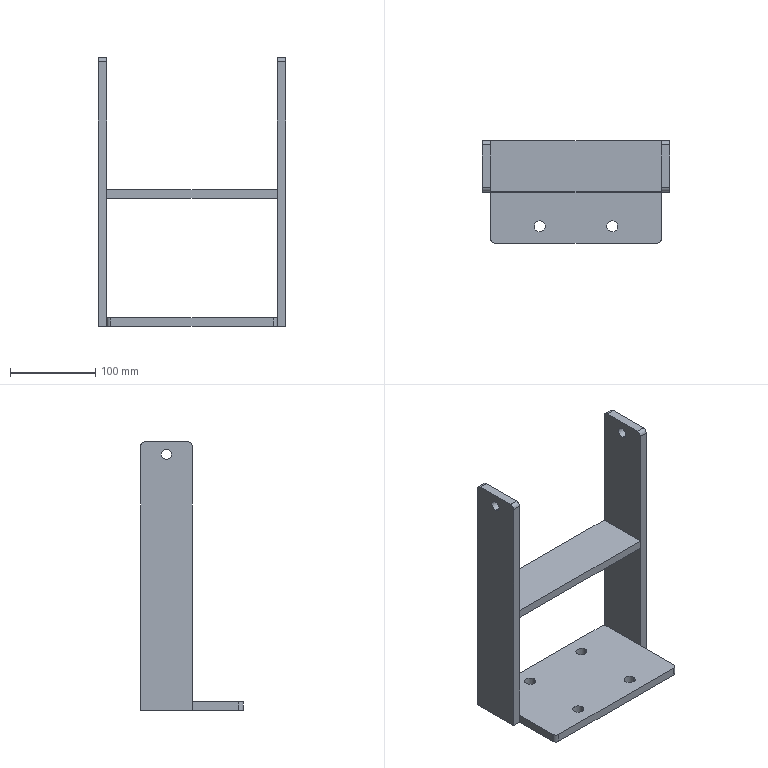Part | 4 solids | 44 faces | box 220 x 120 x 315 mm | volume 730000 mm3 | plane 24 | cylinder 20 | commonest cylinder face diameters 10 x8 13 x8 12 x4
STEP:
#1=CARTESIAN_POINT('',(36.,-40.,10.));
#2=VERTEX_POINT('',#1);
#3=CARTESIAN_POINT('',(49.,-40.,10.));
#4=VERTEX_POINT('',#3);
#5=CARTESIAN_POINT('',(42.5,-40.,10.));
#6=DIRECTION('',(0.,0.,1.));
#7=DIRECTION('',(1.,0.,0.));
#8=AXIS2_PLACEMENT_3D('',#5,#6,#7);
#9=CIRCLE('',#8,6.5);
#10=EDGE_CURVE('',#2,#4,#9,.T.);
#11=ORIENTED_EDGE('',*,*,#10,.T.);
#12=CARTESIAN_POINT('',(49.,-40.,0.));
#13=VERTEX_POINT('',#12);
#14=CARTESIAN_POINT('',(49.,-40.,10.));
#15=DIRECTION('',(0.,0.,-1.));
#16=VECTOR('',#15,1000.);
#17=LINE('',#14,#16);
#18=EDGE_CURVE('',#4,#13,#17,.T.);
#19=ORIENTED_EDGE('',*,*,#18,.T.);
#20=CARTESIAN_POINT('',(36.,-40.,0.));
#21=VERTEX_POINT('',#20);
#22=CARTESIAN_POINT('',(42.5,-40.,0.));
#23=DIRECTION('',(0.,0.,1.));
#24=DIRECTION('',(1.,0.,0.));
#25=AXIS2_PLACEMENT_3D('',#22,#23,#24);
#26=CIRCLE('',#25,6.5);
#27=EDGE_CURVE('',#21,#13,#26,.T.);
#28=ORIENTED_EDGE('',*,*,#27,.F.);
#29=CARTESIAN_POINT('',(36.,-40.,10.));
#30=DIRECTION('',(0.,0.,-1.));
#31=VECTOR('',#30,1000.);
#32=LINE('',#29,#31);
#33=EDGE_CURVE('',#2,#21,#32,.T.);
#34=ORIENTED_EDGE('',*,*,#33,.F.);
#35=EDGE_LOOP('',(#11,#19,#28,#34));
#36=FACE_OUTER_BOUND('',#35,.T.);
#37=CARTESIAN_POINT('',(42.5,-40.,10.));
#38=DIRECTION('',(0.,0.,-1.));
#39=DIRECTION('',(-1.,0.,0.));
#40=AXIS2_PLACEMENT_3D('',#37,#38,#39);
#41=CYLINDRICAL_SURFACE('',#40,6.5);
#42=ADVANCED_FACE('',(#36),#41,.F.);
#43=CARTESIAN_POINT('',(-49.,-40.,10.));
#44=VERTEX_POINT('',#43);
#45=CARTESIAN_POINT('',(-36.,-40.,10.));
#46=VERTEX_POINT('',#45);
#47=CARTESIAN_POINT('',(-42.5,-40.,10.));
#48=DIRECTION('',(0.,0.,1.));
#49=DIRECTION('',(1.,0.,0.));
#50=AXIS2_PLACEMENT_3D('',#47,#48,#49);
#51=CIRCLE('',#50,6.5);
#52=EDGE_CURVE('',#44,#46,#51,.T.);
#53=ORIENTED_EDGE('',*,*,#52,.T.);
#54=CARTESIAN_POINT('',(-36.,-40.,0.));
#55=VERTEX_POINT('',#54);
#56=CARTESIAN_POINT('',(-36.,-40.,10.));
#57=DIRECTION('',(0.,0.,-1.));
#58=VECTOR('',#57,1000.);
#59=LINE('',#56,#58);
#60=EDGE_CURVE('',#46,#55,#59,.T.);
#61=ORIENTED_EDGE('',*,*,#60,.T.);
#62=CARTESIAN_POINT('',(-49.,-40.,0.));
#63=VERTEX_POINT('',#62);
#64=CARTESIAN_POINT('',(-42.5,-40.,0.));
#65=DIRECTION('',(0.,0.,1.));
#66=DIRECTION('',(1.,0.,0.));
#67=AXIS2_PLACEMENT_3D('',#64,#65,#66);
#68=CIRCLE('',#67,6.5);
#69=EDGE_CURVE('',#63,#55,#68,.T.);
#70=ORIENTED_EDGE('',*,*,#69,.F.);
#71=CARTESIAN_POINT('',(-49.,-40.,10.));
#72=DIRECTION('',(0.,0.,-1.));
#73=VECTOR('',#72,1000.);
#74=LINE('',#71,#73);
#75=EDGE_CURVE('',#44,#63,#74,.T.);
#76=ORIENTED_EDGE('',*,*,#75,.F.);
#77=EDGE_LOOP('',(#53,#61,#70,#76));
#78=FACE_OUTER_BOUND('',#77,.T.);
#79=CARTESIAN_POINT('',(-42.5,-40.,10.));
#80=DIRECTION('',(0.,0.,-1.));
#81=DIRECTION('',(-1.,0.,0.));
#82=AXIS2_PLACEMENT_3D('',#79,#80,#81);
#83=CYLINDRICAL_SURFACE('',#82,6.5);
#84=ADVANCED_FACE('',(#78),#83,.F.);
#85=CARTESIAN_POINT('',(36.,40.,10.));
#86=VERTEX_POINT('',#85);
#87=CARTESIAN_POINT('',(49.,40.,10.));
#88=VERTEX_POINT('',#87);
#89=CARTESIAN_POINT('',(42.5,40.,10.));
#90=DIRECTION('',(0.,0.,1.));
#91=DIRECTION('',(1.,0.,0.));
#92=AXIS2_PLACEMENT_3D('',#89,#90,#91);
#93=CIRCLE('',#92,6.5);
#94=EDGE_CURVE('',#86,#88,#93,.T.);
#95=ORIENTED_EDGE('',*,*,#94,.T.);
#96=CARTESIAN_POINT('',(49.,40.,0.));
#97=VERTEX_POINT('',#96);
#98=CARTESIAN_POINT('',(49.,40.,10.));
#99=DIRECTION('',(0.,0.,-1.));
#100=VECTOR('',#99,1000.);
#101=LINE('',#98,#100);
#102=EDGE_CURVE('',#88,#97,#101,.T.);
#103=ORIENTED_EDGE('',*,*,#102,.T.);
#104=CARTESIAN_POINT('',(36.,40.,0.));
#105=VERTEX_POINT('',#104);
#106=CARTESIAN_POINT('',(42.5,40.,0.));
#107=DIRECTION('',(0.,0.,1.));
#108=DIRECTION('',(1.,0.,0.));
#109=AXIS2_PLACEMENT_3D('',#106,#107,#108);
#110=CIRCLE('',#109,6.5);
#111=EDGE_CURVE('',#105,#97,#110,.T.);
#112=ORIENTED_EDGE('',*,*,#111,.F.);
#113=CARTESIAN_POINT('',(36.,40.,10.));
#114=DIRECTION('',(0.,0.,-1.));
#115=VECTOR('',#114,1000.);
#116=LINE('',#113,#115);
#117=EDGE_CURVE('',#86,#105,#116,.T.);
#118=ORIENTED_EDGE('',*,*,#117,.F.);
#119=EDGE_LOOP('',(#95,#103,#112,#118));
#120=FACE_OUTER_BOUND('',#119,.T.);
#121=CARTESIAN_POINT('',(42.5,40.,10.));
#122=DIRECTION('',(0.,0.,-1.));
#123=DIRECTION('',(-1.,0.,0.));
#124=AXIS2_PLACEMENT_3D('',#121,#122,#123);
#125=CYLINDRICAL_SURFACE('',#124,6.5);
#126=ADVANCED_FACE('',(#120),#125,.F.);
#127=CARTESIAN_POINT('',(-49.,40.,10.));
#128=VERTEX_POINT('',#127);
#129=CARTESIAN_POINT('',(-36.,40.,10.));
#130=VERTEX_POINT('',#129);
#131=CARTESIAN_POINT('',(-42.5,40.,10.));
#132=DIRECTION('',(0.,0.,1.));
#133=DIRECTION('',(1.,0.,0.));
#134=AXIS2_PLACEMENT_3D('',#131,#132,#133);
#135=CIRCLE('',#134,6.5);
#136=EDGE_CURVE('',#128,#130,#135,.T.);
#137=ORIENTED_EDGE('',*,*,#136,.T.);
#138=CARTESIAN_POINT('',(-36.,40.,0.));
#139=VERTEX_POINT('',#138);
#140=CARTESIAN_POINT('',(-36.,40.,10.));
#141=DIRECTION('',(0.,0.,-1.));
#142=VECTOR('',#141,1000.);
#143=LINE('',#140,#142);
#144=EDGE_CURVE('',#130,#139,#143,.T.);
#145=ORIENTED_EDGE('',*,*,#144,.T.);
#146=CARTESIAN_POINT('',(-49.,40.,0.));
#147=VERTEX_POINT('',#146);
#148=CARTESIAN_POINT('',(-42.5,40.,0.));
#149=DIRECTION('',(0.,0.,1.));
#150=DIRECTION('',(1.,0.,0.));
#151=AXIS2_PLACEMENT_3D('',#148,#149,#150);
#152=CIRCLE('',#151,6.5);
#153=EDGE_CURVE('',#147,#139,#152,.T.);
#154=ORIENTED_EDGE('',*,*,#153,.F.);
#155=CARTESIAN_POINT('',(-49.,40.,10.));
#156=DIRECTION('',(0.,0.,-1.));
#157=VECTOR('',#156,1000.);
#158=LINE('',#155,#157);
#159=EDGE_CURVE('',#128,#147,#158,.T.);
#160=ORIENTED_EDGE('',*,*,#159,.F.);
#161=EDGE_LOOP('',(#137,#145,#154,#160));
#162=FACE_OUTER_BOUND('',#161,.T.);
#163=CARTESIAN_POINT('',(-42.5,40.,10.));
#164=DIRECTION('',(0.,0.,-1.));
#165=DIRECTION('',(-1.,0.,0.));
#166=AXIS2_PLACEMENT_3D('',#163,#164,#165);
#167=CYLINDRICAL_SURFACE('',#166,6.5);
#168=ADVANCED_FACE('',(#162),#167,.F.);
#169=ORIENTED_EDGE('',*,*,#52,.F.);
#170=CARTESIAN_POINT('',(-42.5,-40.,10.));
#171=DIRECTION('',(0.,0.,1.));
#172=DIRECTION('',(1.,0.,0.));
#173=AXIS2_PLACEMENT_3D('',#170,#171,#172);
#174=CIRCLE('',#173,6.5);
#175=EDGE_CURVE('',#46,#44,#174,.T.);
#176=ORIENTED_EDGE('',*,*,#175,.F.);
#177=EDGE_LOOP('',(#169,#176));
#178=FACE_BOUND('',#177,.T.);
#179=ORIENTED_EDGE('',*,*,#136,.F.);
#180=CARTESIAN_POINT('',(-42.5,40.,10.));
#181=DIRECTION('',(0.,0.,1.));
#182=DIRECTION('',(1.,0.,0.));
#183=AXIS2_PLACEMENT_3D('',#180,#181,#182);
#184=CIRCLE('',#183,6.5);
#185=EDGE_CURVE('',#130,#128,#184,.T.);
#186=ORIENTED_EDGE('',*,*,#185,.F.);
#187=EDGE_LOOP('',(#179,#186));
#188=FACE_BOUND('',#187,.T.);
#189=CARTESIAN_POINT('',(-100.,-55.,10.));
#190=VERTEX_POINT('',#189);
#191=CARTESIAN_POINT('',(-95.,-60.,10.));
#192=VERTEX_POINT('',#191);
#193=CARTESIAN_POINT('',(-95.,-55.,10.));
#194=DIRECTION('',(0.,0.,1.));
#195=DIRECTION('',(1.,0.,0.));
#196=AXIS2_PLACEMENT_3D('',#193,#194,#195);
#197=CIRCLE('',#196,5.);
#198=EDGE_CURVE('',#190,#192,#197,.T.);
#199=ORIENTED_EDGE('',*,*,#198,.T.);
#200=CARTESIAN_POINT('',(95.,-60.,10.));
#201=VERTEX_POINT('',#200);
#202=CARTESIAN_POINT('',(-95.,-60.,10.));
#203=DIRECTION('',(1.,0.,0.));
#204=VECTOR('',#203,1000.);
#205=LINE('',#202,#204);
#206=EDGE_CURVE('',#192,#201,#205,.T.);
#207=ORIENTED_EDGE('',*,*,#206,.T.);
#208=CARTESIAN_POINT('',(100.,-55.,10.));
#209=VERTEX_POINT('',#208);
#210=CARTESIAN_POINT('',(95.,-55.,10.));
#211=DIRECTION('',(0.,0.,1.));
#212=DIRECTION('',(1.,0.,0.));
#213=AXIS2_PLACEMENT_3D('',#210,#211,#212);
#214=CIRCLE('',#213,5.);
#215=EDGE_CURVE('',#201,#209,#214,.T.);
#216=ORIENTED_EDGE('',*,*,#215,.T.);
#217=CARTESIAN_POINT('',(100.,55.,10.));
#218=VERTEX_POINT('',#217);
#219=CARTESIAN_POINT('',(100.,55.,10.));
#220=DIRECTION('',(0.,1.,0.));
#221=VECTOR('',#220,1000.);
#222=LINE('',#219,#221);
#223=EDGE_CURVE('',#209,#218,#222,.T.);
#224=ORIENTED_EDGE('',*,*,#223,.T.);
#225=CARTESIAN_POINT('',(95.,60.,10.));
#226=VERTEX_POINT('',#225);
#227=CARTESIAN_POINT('',(95.,55.,10.));
#228=DIRECTION('',(0.,0.,1.));
#229=DIRECTION('',(-1.,0.,0.));
#230=AXIS2_PLACEMENT_3D('',#227,#228,#229);
#231=CIRCLE('',#230,5.);
#232=EDGE_CURVE('',#218,#226,#231,.T.);
#233=ORIENTED_EDGE('',*,*,#232,.T.);
#234=CARTESIAN_POINT('',(-95.,60.,10.));
#235=VERTEX_POINT('',#234);
#236=CARTESIAN_POINT('',(-95.,60.,10.));
#237=DIRECTION('',(-1.,0.,0.));
#238=VECTOR('',#237,1000.);
#239=LINE('',#236,#238);
#240=EDGE_CURVE('',#226,#235,#239,.T.);
#241=ORIENTED_EDGE('',*,*,#240,.T.);
#242=CARTESIAN_POINT('',(-100.,55.,10.));
#243=VERTEX_POINT('',#242);
#244=CARTESIAN_POINT('',(-95.,55.,10.));
#245=DIRECTION('',(0.,0.,1.));
#246=DIRECTION('',(1.,0.,0.));
#247=AXIS2_PLACEMENT_3D('',#244,#245,#246);
#248=CIRCLE('',#247,5.);
#249=EDGE_CURVE('',#235,#243,#248,.T.);
#250=ORIENTED_EDGE('',*,*,#249,.T.);
#251=CARTESIAN_POINT('',(-100.,55.,10.));
#252=DIRECTION('',(0.,-1.,0.));
#253=VECTOR('',#252,1000.);
#254=LINE('',#251,#253);
#255=EDGE_CURVE('',#243,#190,#254,.T.);
#256=ORIENTED_EDGE('',*,*,#255,.T.);
#257=EDGE_LOOP('',(#199,#207,#216,#224,#233,#241,#250,#256));
#258=FACE_OUTER_BOUND('',#257,.T.);
#259=ORIENTED_EDGE('',*,*,#94,.F.);
#260=CARTESIAN_POINT('',(42.5,40.,10.));
#261=DIRECTION('',(0.,0.,1.));
#262=DIRECTION('',(1.,0.,0.));
#263=AXIS2_PLACEMENT_3D('',#260,#261,#262);
#264=CIRCLE('',#263,6.5);
#265=EDGE_CURVE('',#88,#86,#264,.T.);
#266=ORIENTED_EDGE('',*,*,#265,.F.);
#267=EDGE_LOOP('',(#259,#266));
#268=FACE_BOUND('',#267,.T.);
#269=ORIENTED_EDGE('',*,*,#10,.F.);
#270=CARTESIAN_POINT('',(42.5,-40.,10.));
#271=DIRECTION('',(0.,0.,1.));
#272=DIRECTION('',(1.,0.,0.));
#273=AXIS2_PLACEMENT_3D('',#270,#271,#272);
#274=CIRCLE('',#273,6.5);
#275=EDGE_CURVE('',#4,#2,#274,.T.);
#276=ORIENTED_EDGE('',*,*,#275,.F.);
#277=EDGE_LOOP('',(#269,#276));
#278=FACE_BOUND('',#277,.T.);
#279=CARTESIAN_POINT('',(-95.,-55.,10.));
#280=DIRECTION('',(0.,0.,1.));
#281=DIRECTION('',(1.,0.,0.));
#282=AXIS2_PLACEMENT_3D('',#279,#280,#281);
#283=PLANE('',#282);
#284=ADVANCED_FACE('',(#178,#188,#258,#268,#278),#283,.T.);
#285=CARTESIAN_POINT('',(-100.,-55.,0.));
#286=VERTEX_POINT('',#285);
#287=CARTESIAN_POINT('',(-95.,-60.,0.));
#288=VERTEX_POINT('',#287);
#289=CARTESIAN_POINT('',(-95.,-55.,0.));
#290=DIRECTION('',(0.,0.,1.));
#291=DIRECTION('',(1.,0.,0.));
#292=AXIS2_PLACEMENT_3D('',#289,#290,#291);
#293=CIRCLE('',#292,5.);
#294=EDGE_CURVE('',#286,#288,#293,.T.);
#295=ORIENTED_EDGE('',*,*,#294,.F.);
#296=CARTESIAN_POINT('',(-100.,55.,0.));
#297=VERTEX_POINT('',#296);
#298=CARTESIAN_POINT('',(-100.,55.,0.));
#299=DIRECTION('',(0.,-1.,0.));
#300=VECTOR('',#299,1000.);
#301=LINE('',#298,#300);
#302=EDGE_CURVE('',#297,#286,#301,.T.);
#303=ORIENTED_EDGE('',*,*,#302,.F.);
#304=CARTESIAN_POINT('',(-95.,60.,0.));
#305=VERTEX_POINT('',#304);
#306=CARTESIAN_POINT('',(-95.,55.,0.));
#307=DIRECTION('',(0.,0.,1.));
#308=DIRECTION('',(1.,0.,0.));
#309=AXIS2_PLACEMENT_3D('',#306,#307,#308);
#310=CIRCLE('',#309,5.);
#311=EDGE_CURVE('',#305,#297,#310,.T.);
#312=ORIENTED_EDGE('',*,*,#311,.F.);
#313=CARTESIAN_POINT('',(95.,60.,0.));
#314=VERTEX_POINT('',#313);
#315=CARTESIAN_POINT('',(-95.,60.,0.));
#316=DIRECTION('',(-1.,0.,0.));
#317=VECTOR('',#316,1000.);
#318=LINE('',#315,#317);
#319=EDGE_CURVE('',#314,#305,#318,.T.);
#320=ORIENTED_EDGE('',*,*,#319,.F.);
#321=CARTESIAN_POINT('',(100.,55.,0.));
#322=VERTEX_POINT('',#321);
#323=CARTESIAN_POINT('',(95.,55.,0.));
#324=DIRECTION('',(0.,0.,1.));
#325=DIRECTION('',(-1.,0.,0.));
#326=AXIS2_PLACEMENT_3D('',#323,#324,#325);
#327=CIRCLE('',#326,5.);
#328=EDGE_CURVE('',#322,#314,#327,.T.);
#329=ORIENTED_EDGE('',*,*,#328,.F.);
#330=CARTESIAN_POINT('',(100.,-55.,0.));
#331=VERTEX_POINT('',#330);
#332=CARTESIAN_POINT('',(100.,55.,0.));
#333=DIRECTION('',(0.,1.,0.));
#334=VECTOR('',#333,1000.);
#335=LINE('',#332,#334);
#336=EDGE_CURVE('',#331,#322,#335,.T.);
#337=ORIENTED_EDGE('',*,*,#336,.F.);
#338=CARTESIAN_POINT('',(95.,-60.,0.));
#339=VERTEX_POINT('',#338);
#340=CARTESIAN_POINT('',(95.,-55.,0.));
#341=DIRECTION('',(0.,0.,1.));
#342=DIRECTION('',(1.,0.,0.));
#343=AXIS2_PLACEMENT_3D('',#340,#341,#342);
#344=CIRCLE('',#343,5.);
#345=EDGE_CURVE('',#339,#331,#344,.T.);
#346=ORIENTED_EDGE('',*,*,#345,.F.);
#347=CARTESIAN_POINT('',(-95.,-60.,0.));
#348=DIRECTION('',(1.,0.,0.));
#349=VECTOR('',#348,1000.);
#350=LINE('',#347,#349);
#351=EDGE_CURVE('',#288,#339,#350,.T.);
#352=ORIENTED_EDGE('',*,*,#351,.F.);
#353=EDGE_LOOP('',(#295,#303,#312,#320,#329,#337,#346,#352));
#354=FACE_OUTER_BOUND('',#353,.T.);
#355=ORIENTED_EDGE('',*,*,#153,.T.);
#356=CARTESIAN_POINT('',(-42.5,40.,0.));
#357=DIRECTION('',(0.,0.,1.));
#358=DIRECTION('',(1.,0.,0.));
#359=AXIS2_PLACEMENT_3D('',#356,#357,#358);
#360=CIRCLE('',#359,6.5);
#361=EDGE_CURVE('',#139,#147,#360,.T.);
#362=ORIENTED_EDGE('',*,*,#361,.T.);
#363=EDGE_LOOP('',(#355,#362));
#364=FACE_BOUND('',#363,.T.);
#365=ORIENTED_EDGE('',*,*,#111,.T.);
#366=CARTESIAN_POINT('',(42.5,40.,0.));
#367=DIRECTION('',(0.,0.,1.));
#368=DIRECTION('',(1.,0.,0.));
#369=AXIS2_PLACEMENT_3D('',#366,#367,#368);
#370=CIRCLE('',#369,6.5);
#371=EDGE_CURVE('',#97,#105,#370,.T.);
#372=ORIENTED_EDGE('',*,*,#371,.T.);
#373=EDGE_LOOP('',(#365,#372));
#374=FACE_BOUND('',#373,.T.);
#375=ORIENTED_EDGE('',*,*,#69,.T.);
#376=CARTESIAN_POINT('',(-42.5,-40.,0.));
#377=DIRECTION('',(0.,0.,1.));
#378=DIRECTION('',(1.,0.,0.));
#379=AXIS2_PLACEMENT_3D('',#376,#377,#378);
#380=CIRCLE('',#379,6.5);
#381=EDGE_CURVE('',#55,#63,#380,.T.);
#382=ORIENTED_EDGE('',*,*,#381,.T.);
#383=EDGE_LOOP('',(#375,#382));
#384=FACE_BOUND('',#383,.T.);
#385=ORIENTED_EDGE('',*,*,#27,.T.);
#386=CARTESIAN_POINT('',(42.5,-40.,0.));
#387=DIRECTION('',(0.,0.,1.));
#388=DIRECTION('',(1.,0.,0.));
#389=AXIS2_PLACEMENT_3D('',#386,#387,#388);
#390=CIRCLE('',#389,6.5);
#391=EDGE_CURVE('',#13,#21,#390,.T.);
#392=ORIENTED_EDGE('',*,*,#391,.T.);
#393=EDGE_LOOP('',(#385,#392));
#394=FACE_BOUND('',#393,.T.);
#395=CARTESIAN_POINT('',(-95.,-55.,0.));
#396=DIRECTION('',(0.,0.,1.));
#397=DIRECTION('',(1.,0.,0.));
#398=AXIS2_PLACEMENT_3D('',#395,#396,#397);
#399=PLANE('',#398);
#400=ADVANCED_FACE('',(#354,#364,#374,#384,#394),#399,.F.);
#401=ORIENTED_EDGE('',*,*,#294,.T.);
#402=CARTESIAN_POINT('',(-95.,-60.,10.));
#403=DIRECTION('',(0.,0.,-1.));
#404=VECTOR('',#403,1000.);
#405=LINE('',#402,#404);
#406=EDGE_CURVE('',#192,#288,#405,.T.);
#407=ORIENTED_EDGE('',*,*,#406,.F.);
#408=ORIENTED_EDGE('',*,*,#198,.F.);
#409=CARTESIAN_POINT('',(-100.,-55.,10.));
#410=DIRECTION('',(0.,0.,-1.));
#411=VECTOR('',#410,1000.);
#412=LINE('',#409,#411);
#413=EDGE_CURVE('',#190,#286,#412,.T.);
#414=ORIENTED_EDGE('',*,*,#413,.T.);
#415=EDGE_LOOP('',(#401,#407,#408,#414));
#416=FACE_OUTER_BOUND('',#415,.T.);
#417=CARTESIAN_POINT('',(-95.,-55.,10.));
#418=DIRECTION('',(0.,0.,-1.));
#419=DIRECTION('',(-1.,0.,0.));
#420=AXIS2_PLACEMENT_3D('',#417,#418,#419);
#421=CYLINDRICAL_SURFACE('',#420,5.);
#422=ADVANCED_FACE('',(#416),#421,.T.);
#423=ORIENTED_EDGE('',*,*,#351,.T.);
#424=CARTESIAN_POINT('',(95.,-60.,10.));
#425=DIRECTION('',(0.,0.,-1.));
#426=VECTOR('',#425,1000.);
#427=LINE('',#424,#426);
#428=EDGE_CURVE('',#201,#339,#427,.T.);
#429=ORIENTED_EDGE('',*,*,#428,.F.);
#430=ORIENTED_EDGE('',*,*,#206,.F.);
#431=ORIENTED_EDGE('',*,*,#406,.T.);
#432=EDGE_LOOP('',(#423,#429,#430,#431));
#433=FACE_OUTER_BOUND('',#432,.T.);
#434=CARTESIAN_POINT('',(-95.,-60.,10.));
#435=DIRECTION('',(0.,1.,0.));
#436=DIRECTION('',(0.,0.,1.));
#437=AXIS2_PLACEMENT_3D('',#434,#435,#436);
#438=PLANE('',#437);
#439=ADVANCED_FACE('',(#433),#438,.F.);
#440=ORIENTED_EDGE('',*,*,#345,.T.);
#441=CARTESIAN_POINT('',(100.,-55.,10.));
#442=DIRECTION('',(0.,0.,-1.));
#443=VECTOR('',#442,1000.);
#444=LINE('',#441,#443);
#445=EDGE_CURVE('',#209,#331,#444,.T.);
#446=ORIENTED_EDGE('',*,*,#445,.F.);
#447=ORIENTED_EDGE('',*,*,#215,.F.);
#448=ORIENTED_EDGE('',*,*,#428,.T.);
#449=EDGE_LOOP('',(#440,#446,#447,#448));
#450=FACE_OUTER_BOUND('',#449,.T.);
#451=CARTESIAN_POINT('',(95.,-55.,10.));
#452=DIRECTION('',(0.,0.,-1.));
#453=DIRECTION('',(-1.,0.,0.));
#454=AXIS2_PLACEMENT_3D('',#451,#452,#453);
#455=CYLINDRICAL_SURFACE('',#454,5.);
#456=ADVANCED_FACE('',(#450),#455,.T.);
#457=ORIENTED_EDGE('',*,*,#336,.T.);
#458=CARTESIAN_POINT('',(100.,55.,10.));
#459=DIRECTION('',(0.,0.,-1.));
#460=VECTOR('',#459,1000.);
#461=LINE('',#458,#460);
#462=EDGE_CURVE('',#218,#322,#461,.T.);
#463=ORIENTED_EDGE('',*,*,#462,.F.);
#464=ORIENTED_EDGE('',*,*,#223,.F.);
#465=ORIENTED_EDGE('',*,*,#445,.T.);
#466=EDGE_LOOP('',(#457,#463,#464,#465));
#467=FACE_OUTER_BOUND('',#466,.T.);
#468=CARTESIAN_POINT('',(100.,55.,10.));
#469=DIRECTION('',(-1.,0.,0.));
#470=DIRECTION('',(0.,0.,1.));
#471=AXIS2_PLACEMENT_3D('',#468,#469,#470);
#472=PLANE('',#471);
#473=ADVANCED_FACE('',(#467),#472,.F.);
#474=ORIENTED_EDGE('',*,*,#328,.T.);
#475=CARTESIAN_POINT('',(95.,60.,10.));
#476=DIRECTION('',(0.,0.,-1.));
#477=VECTOR('',#476,1000.);
#478=LINE('',#475,#477);
#479=EDGE_CURVE('',#226,#314,#478,.T.);
#480=ORIENTED_EDGE('',*,*,#479,.F.);
#481=ORIENTED_EDGE('',*,*,#232,.F.);
#482=ORIENTED_EDGE('',*,*,#462,.T.);
#483=EDGE_LOOP('',(#474,#480,#481,#482));
#484=FACE_OUTER_BOUND('',#483,.T.);
#485=CARTESIAN_POINT('',(95.,55.,10.));
#486=DIRECTION('',(0.,0.,-1.));
#487=DIRECTION('',(-1.,0.,0.));
#488=AXIS2_PLACEMENT_3D('',#485,#486,#487);
#489=CYLINDRICAL_SURFACE('',#488,5.);
#490=ADVANCED_FACE('',(#484),#489,.T.);
#491=ORIENTED_EDGE('',*,*,#319,.T.);
#492=CARTESIAN_POINT('',(-95.,60.,10.));
#493=DIRECTION('',(0.,0.,-1.));
#494=VECTOR('',#493,1000.);
#495=LINE('',#492,#494);
#496=EDGE_CURVE('',#235,#305,#495,.T.);
#497=ORIENTED_EDGE('',*,*,#496,.F.);
#498=ORIENTED_EDGE('',*,*,#240,.F.);
#499=ORIENTED_EDGE('',*,*,#479,.T.);
#500=EDGE_LOOP('',(#491,#497,#498,#499));
#501=FACE_OUTER_BOUND('',#500,.T.);
#502=CARTESIAN_POINT('',(-95.,60.,10.));
#503=DIRECTION('',(0.,-1.,0.));
#504=DIRECTION('',(0.,0.,-1.));
#505=AXIS2_PLACEMENT_3D('',#502,#503,#504);
#506=PLANE('',#505);
#507=ADVANCED_FACE('',(#501),#506,.F.);
#508=ORIENTED_EDGE('',*,*,#311,.T.);
#509=CARTESIAN_POINT('',(-100.,55.,10.));
#510=DIRECTION('',(0.,0.,-1.));
#511=VECTOR('',#510,1000.);
#512=LINE('',#509,#511);
#513=EDGE_CURVE('',#243,#297,#512,.T.);
#514=ORIENTED_EDGE('',*,*,#513,.F.);
#515=ORIENTED_EDGE('',*,*,#249,.F.);
#516=ORIENTED_EDGE('',*,*,#496,.T.);
#517=EDGE_LOOP('',(#508,#514,#515,#516));
#518=FACE_OUTER_BOUND('',#517,.T.);
#519=CARTESIAN_POINT('',(-95.,55.,10.));
#520=DIRECTION('',(0.,0.,-1.));
#521=DIRECTION('',(-1.,0.,0.));
#522=AXIS2_PLACEMENT_3D('',#519,#520,#521);
#523=CYLINDRICAL_SURFACE('',#522,5.);
#524=ADVANCED_FACE('',(#518),#523,.T.);
#525=ORIENTED_EDGE('',*,*,#302,.T.);
#526=ORIENTED_EDGE('',*,*,#413,.F.);
#527=ORIENTED_EDGE('',*,*,#255,.F.);
#528=ORIENTED_EDGE('',*,*,#513,.T.);
#529=EDGE_LOOP('',(#525,#526,#527,#528));
#530=FACE_OUTER_BOUND('',#529,.T.);
#531=CARTESIAN_POINT('',(-100.,55.,10.));
#532=DIRECTION('',(1.,0.,0.));
#533=DIRECTION('',(0.,0.,-1.));
#534=AXIS2_PLACEMENT_3D('',#531,#532,#533);
#535=PLANE('',#534);
#536=ADVANCED_FACE('',(#530),#535,.F.);
#537=ORIENTED_EDGE('',*,*,#144,.F.);
#538=ORIENTED_EDGE('',*,*,#185,.T.);
#539=ORIENTED_EDGE('',*,*,#159,.T.);
#540=ORIENTED_EDGE('',*,*,#361,.F.);
#541=EDGE_LOOP('',(#537,#538,#539,#540));
#542=FACE_OUTER_BOUND('',#541,.T.);
#543=CARTESIAN_POINT('',(-42.5,40.,10.));
#544=DIRECTION('',(0.,0.,-1.));
#545=DIRECTION('',(-1.,0.,0.));
#546=AXIS2_PLACEMENT_3D('',#543,#544,#545);
#547=CYLINDRICAL_SURFACE('',#546,6.5);
#548=ADVANCED_FACE('',(#542),#547,.F.);
#549=ORIENTED_EDGE('',*,*,#102,.F.);
#550=ORIENTED_EDGE('',*,*,#265,.T.);
#551=ORIENTED_EDGE('',*,*,#117,.T.);
#552=ORIENTED_EDGE('',*,*,#371,.F.);
#553=EDGE_LOOP('',(#549,#550,#551,#552));
#554=FACE_OUTER_BOUND('',#553,.T.);
#555=CARTESIAN_POINT('',(42.5,40.,10.));
#556=DIRECTION('',(0.,0.,-1.));
#557=DIRECTION('',(-1.,0.,0.));
#558=AXIS2_PLACEMENT_3D('',#555,#556,#557);
#559=CYLINDRICAL_SURFACE('',#558,6.5);
#560=ADVANCED_FACE('',(#554),#559,.F.);
#561=ORIENTED_EDGE('',*,*,#60,.F.);
#562=ORIENTED_EDGE('',*,*,#175,.T.);
#563=ORIENTED_EDGE('',*,*,#75,.T.);
#564=ORIENTED_EDGE('',*,*,#381,.F.);
#565=EDGE_LOOP('',(#561,#562,#563,#564));
#566=FACE_OUTER_BOUND('',#565,.T.);
#567=CARTESIAN_POINT('',(-42.5,-40.,10.));
#568=DIRECTION('',(0.,0.,-1.));
#569=DIRECTION('',(-1.,0.,0.));
#570=AXIS2_PLACEMENT_3D('',#567,#568,#569);
#571=CYLINDRICAL_SURFACE('',#570,6.5);
#572=ADVANCED_FACE('',(#566),#571,.F.);
#573=ORIENTED_EDGE('',*,*,#18,.F.);
#574=ORIENTED_EDGE('',*,*,#275,.T.);
#575=ORIENTED_EDGE('',*,*,#33,.T.);
#576=ORIENTED_EDGE('',*,*,#391,.F.);
#577=EDGE_LOOP('',(#573,#574,#575,#576));
#578=FACE_OUTER_BOUND('',#577,.T.);
#579=CARTESIAN_POINT('',(42.5,-40.,10.));
#580=DIRECTION('',(0.,0.,-1.));
#581=DIRECTION('',(-1.,0.,0.));
#582=AXIS2_PLACEMENT_3D('',#579,#580,#581);
#583=CYLINDRICAL_SURFACE('',#582,6.5);
#584=ADVANCED_FACE('',(#578),#583,.F.);
#585=CLOSED_SHELL('',(#42,#84,#126,#168,#284,#400,#422,#439,#456,#473,#490,#507,#524,#536,#548,#560,#572,#584));
#586=MANIFOLD_SOLID_BREP('',#585);
#587=CARTESIAN_POINT('',(-110.,30.,294.));
#588=VERTEX_POINT('',#587);
#589=CARTESIAN_POINT('',(-110.,30.,306.));
#590=VERTEX_POINT('',#589);
#591=CARTESIAN_POINT('',(-110.,30.,300.));
#592=DIRECTION('',(-1.,0.,0.));
#593=DIRECTION('',(0.,0.,1.));
#594=AXIS2_PLACEMENT_3D('',#591,#592,#593);
#595=CIRCLE('',#594,6.);
#596=EDGE_CURVE('',#588,#590,#595,.T.);
#597=ORIENTED_EDGE('',*,*,#596,.T.);
#598=CARTESIAN_POINT('',(-100.,30.,306.));
#599=VERTEX_POINT('',#598);
#600=CARTESIAN_POINT('',(-110.,30.,306.));
#601=DIRECTION('',(1.,0.,0.));
#602=VECTOR('',#601,1000.);
#603=LINE('',#600,#602);
#604=EDGE_CURVE('',#590,#599,#603,.T.);
#605=ORIENTED_EDGE('',*,*,#604,.T.);
#606=CARTESIAN_POINT('',(-100.,30.,294.));
#607=VERTEX_POINT('',#606);
#608=CARTESIAN_POINT('',(-100.,30.,300.));
#609=DIRECTION('',(-1.,0.,0.));
#610=DIRECTION('',(0.,0.,1.));
#611=AXIS2_PLACEMENT_3D('',#608,#609,#610);
#612=CIRCLE('',#611,6.);
#613=EDGE_CURVE('',#607,#599,#612,.T.);
#614=ORIENTED_EDGE('',*,*,#613,.F.);
#615=CARTESIAN_POINT('',(-110.,30.,294.));
#616=DIRECTION('',(1.,0.,0.));
#617=VECTOR('',#616,1000.);
#618=LINE('',#615,#617);
#619=EDGE_CURVE('',#588,#607,#618,.T.);
#620=ORIENTED_EDGE('',*,*,#619,.F.);
#621=EDGE_LOOP('',(#597,#605,#614,#620));
#622=FACE_OUTER_BOUND('',#621,.T.);
#623=CARTESIAN_POINT('',(-110.,30.,300.));
#624=DIRECTION('',(1.,0.,0.));
#625=DIRECTION('',(0.,0.,-1.));
#626=AXIS2_PLACEMENT_3D('',#623,#624,#625);
#627=CYLINDRICAL_SURFACE('',#626,6.);
#628=ADVANCED_FACE('',(#622),#627,.F.);
#629=CARTESIAN_POINT('',(-110.,0.,0.));
#630=VERTEX_POINT('',#629);
#631=CARTESIAN_POINT('',(-110.,0.,310.));
#632=VERTEX_POINT('',#631);
#633=CARTESIAN_POINT('',(-110.,0.,0.));
#634=DIRECTION('',(0.,0.,1.));
#635=VECTOR('',#634,1000.);
#636=LINE('',#633,#635);
#637=EDGE_CURVE('',#630,#632,#636,.T.);
#638=ORIENTED_EDGE('',*,*,#637,.T.);
#639=CARTESIAN_POINT('',(-110.,5.,315.));
#640=VERTEX_POINT('',#639);
#641=CARTESIAN_POINT('',(-110.,5.,310.));
#642=DIRECTION('',(-1.,0.,0.));
#643=DIRECTION('',(0.,0.,-1.));
#644=AXIS2_PLACEMENT_3D('',#641,#642,#643);
#645=CIRCLE('',#644,5.);
#646=EDGE_CURVE('',#632,#640,#645,.T.);
#647=ORIENTED_EDGE('',*,*,#646,.T.);
#648=CARTESIAN_POINT('',(-110.,55.,315.));
#649=VERTEX_POINT('',#648);
#650=CARTESIAN_POINT('',(-110.,60.,315.));
#651=DIRECTION('',(0.,1.,0.));
#652=VECTOR('',#651,1000.);
#653=LINE('',#650,#652);
#654=EDGE_CURVE('',#640,#649,#653,.T.);
#655=ORIENTED_EDGE('',*,*,#654,.T.);
#656=CARTESIAN_POINT('',(-110.,60.,310.));
#657=VERTEX_POINT('',#656);
#658=CARTESIAN_POINT('',(-110.,55.,310.));
#659=DIRECTION('',(-1.,0.,0.));
#660=DIRECTION('',(0.,0.,-1.));
#661=AXIS2_PLACEMENT_3D('',#658,#659,#660);
#662=CIRCLE('',#661,5.);
#663=EDGE_CURVE('',#649,#657,#662,.T.);
#664=ORIENTED_EDGE('',*,*,#663,.T.);
#665=CARTESIAN_POINT('',(-110.,60.,0.));
#666=VERTEX_POINT('',#665);
#667=CARTESIAN_POINT('',(-110.,60.,0.));
#668=DIRECTION('',(0.,0.,-1.));
#669=VECTOR('',#668,1000.);
#670=LINE('',#667,#669);
#671=EDGE_CURVE('',#657,#666,#670,.T.);
#672=ORIENTED_EDGE('',*,*,#671,.T.);
#673=CARTESIAN_POINT('',(-110.,60.,0.));
#674=DIRECTION('',(0.,-1.,0.));
#675=VECTOR('',#674,1000.);
#676=LINE('',#673,#675);
#677=EDGE_CURVE('',#666,#630,#676,.T.);
#678=ORIENTED_EDGE('',*,*,#677,.T.);
#679=EDGE_LOOP('',(#638,#647,#655,#664,#672,#678));
#680=FACE_OUTER_BOUND('',#679,.T.);
#681=ORIENTED_EDGE('',*,*,#596,.F.);
#682=CARTESIAN_POINT('',(-110.,30.,300.));
#683=DIRECTION('',(-1.,0.,0.));
#684=DIRECTION('',(0.,0.,1.));
#685=AXIS2_PLACEMENT_3D('',#682,#683,#684);
#686=CIRCLE('',#685,6.);
#687=EDGE_CURVE('',#590,#588,#686,.T.);
#688=ORIENTED_EDGE('',*,*,#687,.F.);
#689=EDGE_LOOP('',(#681,#688));
#690=FACE_BOUND('',#689,.T.);
#691=CARTESIAN_POINT('',(-110.,0.,0.));
#692=DIRECTION('',(1.,0.,0.));
#693=DIRECTION('',(0.,0.,-1.));
#694=AXIS2_PLACEMENT_3D('',#691,#692,#693);
#695=PLANE('',#694);
#696=ADVANCED_FACE('',(#680,#690),#695,.F.);
#697=CARTESIAN_POINT('',(-100.,5.,315.));
#698=VERTEX_POINT('',#697);
#699=CARTESIAN_POINT('',(-100.,55.,315.));
#700=VERTEX_POINT('',#699);
#701=CARTESIAN_POINT('',(-100.,60.,315.));
#702=DIRECTION('',(0.,1.,0.));
#703=VECTOR('',#702,1000.);
#704=LINE('',#701,#703);
#705=EDGE_CURVE('',#698,#700,#704,.T.);
#706=ORIENTED_EDGE('',*,*,#705,.F.);
#707=CARTESIAN_POINT('',(-100.,0.,310.));
#708=VERTEX_POINT('',#707);
#709=CARTESIAN_POINT('',(-100.,5.,310.));
#710=DIRECTION('',(1.,0.,0.));
#711=DIRECTION('',(0.,0.,-1.));
#712=AXIS2_PLACEMENT_3D('',#709,#710,#711);
#713=CIRCLE('',#712,5.);
#714=EDGE_CURVE('',#698,#708,#713,.T.);
#715=ORIENTED_EDGE('',*,*,#714,.T.);
#716=CARTESIAN_POINT('',(-100.,0.,0.));
#717=VERTEX_POINT('',#716);
#718=CARTESIAN_POINT('',(-100.,0.,0.));
#719=DIRECTION('',(0.,0.,1.));
#720=VECTOR('',#719,1000.);
#721=LINE('',#718,#720);
#722=EDGE_CURVE('',#717,#708,#721,.T.);
#723=ORIENTED_EDGE('',*,*,#722,.F.);
#724=CARTESIAN_POINT('',(-100.,60.,0.));
#725=VERTEX_POINT('',#724);
#726=CARTESIAN_POINT('',(-100.,60.,0.));
#727=DIRECTION('',(0.,-1.,0.));
#728=VECTOR('',#727,1000.);
#729=LINE('',#726,#728);
#730=EDGE_CURVE('',#725,#717,#729,.T.);
#731=ORIENTED_EDGE('',*,*,#730,.F.);
#732=CARTESIAN_POINT('',(-100.,60.,310.));
#733=VERTEX_POINT('',#732);
#734=CARTESIAN_POINT('',(-100.,60.,0.));
#735=DIRECTION('',(0.,0.,-1.));
#736=VECTOR('',#735,1000.);
#737=LINE('',#734,#736);
#738=EDGE_CURVE('',#733,#725,#737,.T.);
#739=ORIENTED_EDGE('',*,*,#738,.F.);
#740=CARTESIAN_POINT('',(-100.,55.,310.));
#741=DIRECTION('',(1.,0.,0.));
#742=DIRECTION('',(0.,0.,-1.));
#743=AXIS2_PLACEMENT_3D('',#740,#741,#742);
#744=CIRCLE('',#743,5.);
#745=EDGE_CURVE('',#733,#700,#744,.T.);
#746=ORIENTED_EDGE('',*,*,#745,.T.);
#747=EDGE_LOOP('',(#706,#715,#723,#731,#739,#746));
#748=FACE_OUTER_BOUND('',#747,.T.);
#749=ORIENTED_EDGE('',*,*,#613,.T.);
#750=CARTESIAN_POINT('',(-100.,30.,300.));
#751=DIRECTION('',(-1.,0.,0.));
#752=DIRECTION('',(0.,0.,1.));
#753=AXIS2_PLACEMENT_3D('',#750,#751,#752);
#754=CIRCLE('',#753,6.);
#755=EDGE_CURVE('',#599,#607,#754,.T.);
#756=ORIENTED_EDGE('',*,*,#755,.T.);
#757=EDGE_LOOP('',(#749,#756));
#758=FACE_BOUND('',#757,.T.);
#759=CARTESIAN_POINT('',(-100.,0.,0.));
#760=DIRECTION('',(1.,0.,0.));
#761=DIRECTION('',(0.,0.,-1.));
#762=AXIS2_PLACEMENT_3D('',#759,#760,#761);
#763=PLANE('',#762);
#764=ADVANCED_FACE('',(#748,#758),#763,.T.);
#765=ORIENTED_EDGE('',*,*,#671,.F.);
#766=CARTESIAN_POINT('',(-110.,60.,310.));
#767=DIRECTION('',(1.,0.,0.));
#768=VECTOR('',#767,1000.);
#769=LINE('',#766,#768);
#770=EDGE_CURVE('',#657,#733,#769,.T.);
#771=ORIENTED_EDGE('',*,*,#770,.T.);
#772=ORIENTED_EDGE('',*,*,#738,.T.);
#773=CARTESIAN_POINT('',(-110.,60.,0.));
#774=DIRECTION('',(1.,0.,0.));
#775=VECTOR('',#774,1000.);
#776=LINE('',#773,#775);
#777=EDGE_CURVE('',#666,#725,#776,.T.);
#778=ORIENTED_EDGE('',*,*,#777,.F.);
#779=EDGE_LOOP('',(#765,#771,#772,#778));
#780=FACE_OUTER_BOUND('',#779,.T.);
#781=CARTESIAN_POINT('',(-110.,60.,0.));
#782=DIRECTION('',(0.,-1.,0.));
#783=DIRECTION('',(0.,0.,-1.));
#784=AXIS2_PLACEMENT_3D('',#781,#782,#783);
#785=PLANE('',#784);
#786=ADVANCED_FACE('',(#780),#785,.F.);
#787=ORIENTED_EDGE('',*,*,#730,.T.);
#788=CARTESIAN_POINT('',(-110.,0.,0.));
#789=DIRECTION('',(1.,0.,0.));
#790=VECTOR('',#789,1000.);
#791=LINE('',#788,#790);
#792=EDGE_CURVE('',#630,#717,#791,.T.);
#793=ORIENTED_EDGE('',*,*,#792,.F.);
#794=ORIENTED_EDGE('',*,*,#677,.F.);
#795=ORIENTED_EDGE('',*,*,#777,.T.);
#796=EDGE_LOOP('',(#787,#793,#794,#795));
#797=FACE_OUTER_BOUND('',#796,.T.);
#798=CARTESIAN_POINT('',(-110.,60.,0.));
#799=DIRECTION('',(0.,0.,1.));
#800=DIRECTION('',(1.,0.,0.));
#801=AXIS2_PLACEMENT_3D('',#798,#799,#800);
#802=PLANE('',#801);
#803=ADVANCED_FACE('',(#797),#802,.F.);
#804=ORIENTED_EDGE('',*,*,#722,.T.);
#805=CARTESIAN_POINT('',(-110.,0.,310.));
#806=DIRECTION('',(-1.,0.,0.));
#807=VECTOR('',#806,1000.);
#808=LINE('',#805,#807);
#809=EDGE_CURVE('',#708,#632,#808,.T.);
#810=ORIENTED_EDGE('',*,*,#809,.T.);
#811=ORIENTED_EDGE('',*,*,#637,.F.);
#812=ORIENTED_EDGE('',*,*,#792,.T.);
#813=EDGE_LOOP('',(#804,#810,#811,#812));
#814=FACE_OUTER_BOUND('',#813,.T.);
#815=CARTESIAN_POINT('',(-110.,0.,0.));
#816=DIRECTION('',(0.,1.,0.));
#817=DIRECTION('',(0.,0.,1.));
#818=AXIS2_PLACEMENT_3D('',#815,#816,#817);
#819=PLANE('',#818);
#820=ADVANCED_FACE('',(#814),#819,.F.);
#821=ORIENTED_EDGE('',*,*,#654,.F.);
#822=CARTESIAN_POINT('',(-110.,5.,315.));
#823=DIRECTION('',(1.,0.,0.));
#824=VECTOR('',#823,1000.);
#825=LINE('',#822,#824);
#826=EDGE_CURVE('',#640,#698,#825,.T.);
#827=ORIENTED_EDGE('',*,*,#826,.T.);
#828=ORIENTED_EDGE('',*,*,#705,.T.);
#829=CARTESIAN_POINT('',(-110.,55.,315.));
#830=DIRECTION('',(-1.,0.,0.));
#831=VECTOR('',#830,1000.);
#832=LINE('',#829,#831);
#833=EDGE_CURVE('',#700,#649,#832,.T.);
#834=ORIENTED_EDGE('',*,*,#833,.T.);
#835=EDGE_LOOP('',(#821,#827,#828,#834));
#836=FACE_OUTER_BOUND('',#835,.T.);
#837=CARTESIAN_POINT('',(-110.,60.,315.));
#838=DIRECTION('',(0.,0.,-1.));
#839=DIRECTION('',(-1.,0.,0.));
#840=AXIS2_PLACEMENT_3D('',#837,#838,#839);
#841=PLANE('',#840);
#842=ADVANCED_FACE('',(#836),#841,.F.);
#843=ORIENTED_EDGE('',*,*,#604,.F.);
#844=ORIENTED_EDGE('',*,*,#687,.T.);
#845=ORIENTED_EDGE('',*,*,#619,.T.);
#846=ORIENTED_EDGE('',*,*,#755,.F.);
#847=EDGE_LOOP('',(#843,#844,#845,#846));
#848=FACE_OUTER_BOUND('',#847,.T.);
#849=CARTESIAN_POINT('',(-110.,30.,300.));
#850=DIRECTION('',(1.,0.,0.));
#851=DIRECTION('',(0.,0.,-1.));
#852=AXIS2_PLACEMENT_3D('',#849,#850,#851);
#853=CYLINDRICAL_SURFACE('',#852,6.);
#854=ADVANCED_FACE('',(#848),#853,.F.);
#855=ORIENTED_EDGE('',*,*,#646,.F.);
#856=ORIENTED_EDGE('',*,*,#809,.F.);
#857=ORIENTED_EDGE('',*,*,#714,.F.);
#858=ORIENTED_EDGE('',*,*,#826,.F.);
#859=EDGE_LOOP('',(#855,#856,#857,#858));
#860=FACE_OUTER_BOUND('',#859,.T.);
#861=CARTESIAN_POINT('',(-110.,5.,310.));
#862=DIRECTION('',(1.,0.,0.));
#863=DIRECTION('',(0.,0.,-1.));
#864=AXIS2_PLACEMENT_3D('',#861,#862,#863);
#865=CYLINDRICAL_SURFACE('',#864,5.);
#866=ADVANCED_FACE('',(#860),#865,.T.);
#867=ORIENTED_EDGE('',*,*,#663,.F.);
#868=ORIENTED_EDGE('',*,*,#833,.F.);
#869=ORIENTED_EDGE('',*,*,#745,.F.);
#870=ORIENTED_EDGE('',*,*,#770,.F.);
#871=EDGE_LOOP('',(#867,#868,#869,#870));
#872=FACE_OUTER_BOUND('',#871,.T.);
#873=CARTESIAN_POINT('',(-110.,55.,310.));
#874=DIRECTION('',(1.,0.,0.));
#875=DIRECTION('',(0.,0.,-1.));
#876=AXIS2_PLACEMENT_3D('',#873,#874,#875);
#877=CYLINDRICAL_SURFACE('',#876,5.);
#878=ADVANCED_FACE('',(#872),#877,.T.);
#879=CLOSED_SHELL('',(#628,#696,#764,#786,#803,#820,#842,#854,#866,#878));
#880=MANIFOLD_SOLID_BREP('',#879);
#881=CARTESIAN_POINT('',(110.,30.,306.));
#882=VERTEX_POINT('',#881);
#883=CARTESIAN_POINT('',(110.,30.,294.));
#884=VERTEX_POINT('',#883);
#885=CARTESIAN_POINT('',(110.,30.,300.));
#886=DIRECTION('',(-1.,0.,0.));
#887=DIRECTION('',(0.,0.,1.));
#888=AXIS2_PLACEMENT_3D('',#885,#886,#887);
#889=CIRCLE('',#888,6.);
#890=EDGE_CURVE('',#882,#884,#889,.T.);
#891=ORIENTED_EDGE('',*,*,#890,.F.);
#892=CARTESIAN_POINT('',(100.,30.,306.));
#893=VERTEX_POINT('',#892);
#894=CARTESIAN_POINT('',(110.,30.,306.));
#895=DIRECTION('',(-1.,0.,0.));
#896=VECTOR('',#895,1000.);
#897=LINE('',#894,#896);
#898=EDGE_CURVE('',#882,#893,#897,.T.);
#899=ORIENTED_EDGE('',*,*,#898,.T.);
#900=CARTESIAN_POINT('',(100.,30.,294.));
#901=VERTEX_POINT('',#900);
#902=CARTESIAN_POINT('',(100.,30.,300.));
#903=DIRECTION('',(-1.,0.,0.));
#904=DIRECTION('',(0.,0.,1.));
#905=AXIS2_PLACEMENT_3D('',#902,#903,#904);
#906=CIRCLE('',#905,6.);
#907=EDGE_CURVE('',#893,#901,#906,.T.);
#908=ORIENTED_EDGE('',*,*,#907,.T.);
#909=CARTESIAN_POINT('',(110.,30.,294.));
#910=DIRECTION('',(-1.,0.,0.));
#911=VECTOR('',#910,1000.);
#912=LINE('',#909,#911);
#913=EDGE_CURVE('',#884,#901,#912,.T.);
#914=ORIENTED_EDGE('',*,*,#913,.F.);
#915=EDGE_LOOP('',(#891,#899,#908,#914));
#916=FACE_OUTER_BOUND('',#915,.T.);
#917=CARTESIAN_POINT('',(110.,30.,300.));
#918=DIRECTION('',(-1.,0.,0.));
#919=DIRECTION('',(0.,0.,-1.));
#920=AXIS2_PLACEMENT_3D('',#917,#918,#919);
#921=CYLINDRICAL_SURFACE('',#920,6.);
#922=ADVANCED_FACE('',(#916),#921,.F.);
#923=CARTESIAN_POINT('',(110.,5.,315.));
#924=VERTEX_POINT('',#923);
#925=CARTESIAN_POINT('',(110.,55.,315.));
#926=VERTEX_POINT('',#925);
#927=CARTESIAN_POINT('',(110.,60.,315.));
#928=DIRECTION('',(0.,1.,0.));
#929=VECTOR('',#928,1000.);
#930=LINE('',#927,#929);
#931=EDGE_CURVE('',#924,#926,#930,.T.);
#932=ORIENTED_EDGE('',*,*,#931,.F.);
#933=CARTESIAN_POINT('',(110.,0.,310.));
#934=VERTEX_POINT('',#933);
#935=CARTESIAN_POINT('',(110.,5.,310.));
#936=DIRECTION('',(1.,0.,0.));
#937=DIRECTION('',(0.,0.,1.));
#938=AXIS2_PLACEMENT_3D('',#935,#936,#937);
#939=CIRCLE('',#938,5.);
#940=EDGE_CURVE('',#924,#934,#939,.T.);
#941=ORIENTED_EDGE('',*,*,#940,.T.);
#942=CARTESIAN_POINT('',(110.,0.,0.));
#943=VERTEX_POINT('',#942);
#944=CARTESIAN_POINT('',(110.,0.,0.));
#945=DIRECTION('',(0.,0.,1.));
#946=VECTOR('',#945,1000.);
#947=LINE('',#944,#946);
#948=EDGE_CURVE('',#943,#934,#947,.T.);
#949=ORIENTED_EDGE('',*,*,#948,.F.);
#950=CARTESIAN_POINT('',(110.,60.,0.));
#951=VERTEX_POINT('',#950);
#952=CARTESIAN_POINT('',(110.,60.,0.));
#953=DIRECTION('',(0.,-1.,0.));
#954=VECTOR('',#953,1000.);
#955=LINE('',#952,#954);
#956=EDGE_CURVE('',#951,#943,#955,.T.);
#957=ORIENTED_EDGE('',*,*,#956,.F.);
#958=CARTESIAN_POINT('',(110.,60.,310.));
#959=VERTEX_POINT('',#958);
#960=CARTESIAN_POINT('',(110.,60.,0.));
#961=DIRECTION('',(0.,0.,-1.));
#962=VECTOR('',#961,1000.);
#963=LINE('',#960,#962);
#964=EDGE_CURVE('',#959,#951,#963,.T.);
#965=ORIENTED_EDGE('',*,*,#964,.F.);
#966=CARTESIAN_POINT('',(110.,55.,310.));
#967=DIRECTION('',(1.,0.,0.));
#968=DIRECTION('',(0.,0.,1.));
#969=AXIS2_PLACEMENT_3D('',#966,#967,#968);
#970=CIRCLE('',#969,5.);
#971=EDGE_CURVE('',#959,#926,#970,.T.);
#972=ORIENTED_EDGE('',*,*,#971,.T.);
#973=EDGE_LOOP('',(#932,#941,#949,#957,#965,#972));
#974=FACE_OUTER_BOUND('',#973,.T.);
#975=CARTESIAN_POINT('',(110.,30.,300.));
#976=DIRECTION('',(-1.,0.,0.));
#977=DIRECTION('',(0.,0.,1.));
#978=AXIS2_PLACEMENT_3D('',#975,#976,#977);
#979=CIRCLE('',#978,6.);
#980=EDGE_CURVE('',#884,#882,#979,.T.);
#981=ORIENTED_EDGE('',*,*,#980,.T.);
#982=ORIENTED_EDGE('',*,*,#890,.T.);
#983=EDGE_LOOP('',(#981,#982));
#984=FACE_BOUND('',#983,.T.);
#985=CARTESIAN_POINT('',(110.,0.,0.));
#986=DIRECTION('',(-1.,0.,0.));
#987=DIRECTION('',(0.,0.,-1.));
#988=AXIS2_PLACEMENT_3D('',#985,#986,#987);
#989=PLANE('',#988);
#990=ADVANCED_FACE('',(#974,#984),#989,.F.);
#991=CARTESIAN_POINT('',(100.,0.,0.));
#992=VERTEX_POINT('',#991);
#993=CARTESIAN_POINT('',(100.,0.,310.));
#994=VERTEX_POINT('',#993);
#995=CARTESIAN_POINT('',(100.,0.,0.));
#996=DIRECTION('',(0.,0.,1.));
#997=VECTOR('',#996,1000.);
#998=LINE('',#995,#997);
#999=EDGE_CURVE('',#992,#994,#998,.T.);
#1000=ORIENTED_EDGE('',*,*,#999,.T.);
#1001=CARTESIAN_POINT('',(100.,5.,315.));
#1002=VERTEX_POINT('',#1001);
#1003=CARTESIAN_POINT('',(100.,5.,310.));
#1004=DIRECTION('',(-1.,0.,0.));
#1005=DIRECTION('',(0.,0.,1.));
#1006=AXIS2_PLACEMENT_3D('',#1003,#1004,#1005);
#1007=CIRCLE('',#1006,5.);
#1008=EDGE_CURVE('',#994,#1002,#1007,.T.);
#1009=ORIENTED_EDGE('',*,*,#1008,.T.);
#1010=CARTESIAN_POINT('',(100.,55.,315.));
#1011=VERTEX_POINT('',#1010);
#1012=CARTESIAN_POINT('',(100.,60.,315.));
#1013=DIRECTION('',(0.,1.,0.));
#1014=VECTOR('',#1013,1000.);
#1015=LINE('',#1012,#1014);
#1016=EDGE_CURVE('',#1002,#1011,#1015,.T.);
#1017=ORIENTED_EDGE('',*,*,#1016,.T.);
#1018=CARTESIAN_POINT('',(100.,60.,310.));
#1019=VERTEX_POINT('',#1018);
#1020=CARTESIAN_POINT('',(100.,55.,310.));
#1021=DIRECTION('',(-1.,0.,0.));
#1022=DIRECTION('',(0.,0.,1.));
#1023=AXIS2_PLACEMENT_3D('',#1020,#1021,#1022);
#1024=CIRCLE('',#1023,5.);
#1025=EDGE_CURVE('',#1011,#1019,#1024,.T.);
#1026=ORIENTED_EDGE('',*,*,#1025,.T.);
#1027=CARTESIAN_POINT('',(100.,60.,0.));
#1028=VERTEX_POINT('',#1027);
#1029=CARTESIAN_POINT('',(100.,60.,0.));
#1030=DIRECTION('',(0.,0.,-1.));
#1031=VECTOR('',#1030,1000.);
#1032=LINE('',#1029,#1031);
#1033=EDGE_CURVE('',#1019,#1028,#1032,.T.);
#1034=ORIENTED_EDGE('',*,*,#1033,.T.);
#1035=CARTESIAN_POINT('',(100.,60.,0.));
#1036=DIRECTION('',(0.,-1.,0.));
#1037=VECTOR('',#1036,1000.);
#1038=LINE('',#1035,#1037);
#1039=EDGE_CURVE('',#1028,#992,#1038,.T.);
#1040=ORIENTED_EDGE('',*,*,#1039,.T.);
#1041=EDGE_LOOP('',(#1000,#1009,#1017,#1026,#1034,#1040));
#1042=FACE_OUTER_BOUND('',#1041,.T.);
#1043=CARTESIAN_POINT('',(100.,30.,300.));
#1044=DIRECTION('',(-1.,0.,0.));
#1045=DIRECTION('',(0.,0.,1.));
#1046=AXIS2_PLACEMENT_3D('',#1043,#1044,#1045);
#1047=CIRCLE('',#1046,6.);
#1048=EDGE_CURVE('',#901,#893,#1047,.T.);
#1049=ORIENTED_EDGE('',*,*,#1048,.F.);
#1050=ORIENTED_EDGE('',*,*,#907,.F.);
#1051=EDGE_LOOP('',(#1049,#1050));
#1052=FACE_BOUND('',#1051,.T.);
#1053=CARTESIAN_POINT('',(100.,0.,0.));
#1054=DIRECTION('',(-1.,0.,0.));
#1055=DIRECTION('',(0.,0.,-1.));
#1056=AXIS2_PLACEMENT_3D('',#1053,#1054,#1055);
#1057=PLANE('',#1056);
#1058=ADVANCED_FACE('',(#1042,#1052),#1057,.T.);
#1059=ORIENTED_EDGE('',*,*,#1033,.F.);
#1060=CARTESIAN_POINT('',(110.,60.,310.));
#1061=DIRECTION('',(1.,0.,0.));
#1062=VECTOR('',#1061,1000.);
#1063=LINE('',#1060,#1062);
#1064=EDGE_CURVE('',#1019,#959,#1063,.T.);
#1065=ORIENTED_EDGE('',*,*,#1064,.T.);
#1066=ORIENTED_EDGE('',*,*,#964,.T.);
#1067=CARTESIAN_POINT('',(110.,60.,0.));
#1068=DIRECTION('',(-1.,0.,0.));
#1069=VECTOR('',#1068,1000.);
#1070=LINE('',#1067,#1069);
#1071=EDGE_CURVE('',#951,#1028,#1070,.T.);
#1072=ORIENTED_EDGE('',*,*,#1071,.T.);
#1073=EDGE_LOOP('',(#1059,#1065,#1066,#1072));
#1074=FACE_OUTER_BOUND('',#1073,.T.);
#1075=CARTESIAN_POINT('',(110.,60.,0.));
#1076=DIRECTION('',(0.,-1.,0.));
#1077=DIRECTION('',(0.,0.,-1.));
#1078=AXIS2_PLACEMENT_3D('',#1075,#1076,#1077);
#1079=PLANE('',#1078);
#1080=ADVANCED_FACE('',(#1074),#1079,.F.);
#1081=ORIENTED_EDGE('',*,*,#1039,.F.);
#1082=ORIENTED_EDGE('',*,*,#1071,.F.);
#1083=ORIENTED_EDGE('',*,*,#956,.T.);
#1084=CARTESIAN_POINT('',(110.,0.,0.));
#1085=DIRECTION('',(-1.,0.,0.));
#1086=VECTOR('',#1085,1000.);
#1087=LINE('',#1084,#1086);
#1088=EDGE_CURVE('',#943,#992,#1087,.T.);
#1089=ORIENTED_EDGE('',*,*,#1088,.T.);
#1090=EDGE_LOOP('',(#1081,#1082,#1083,#1089));
#1091=FACE_OUTER_BOUND('',#1090,.T.);
#1092=CARTESIAN_POINT('',(110.,60.,0.));
#1093=DIRECTION('',(0.,0.,1.));
#1094=DIRECTION('',(-1.,0.,0.));
#1095=AXIS2_PLACEMENT_3D('',#1092,#1093,#1094);
#1096=PLANE('',#1095);
#1097=ADVANCED_FACE('',(#1091),#1096,.F.);
#1098=ORIENTED_EDGE('',*,*,#948,.T.);
#1099=CARTESIAN_POINT('',(110.,0.,310.));
#1100=DIRECTION('',(-1.,0.,0.));
#1101=VECTOR('',#1100,1000.);
#1102=LINE('',#1099,#1101);
#1103=EDGE_CURVE('',#934,#994,#1102,.T.);
#1104=ORIENTED_EDGE('',*,*,#1103,.T.);
#1105=ORIENTED_EDGE('',*,*,#999,.F.);
#1106=ORIENTED_EDGE('',*,*,#1088,.F.);
#1107=EDGE_LOOP('',(#1098,#1104,#1105,#1106));
#1108=FACE_OUTER_BOUND('',#1107,.T.);
#1109=CARTESIAN_POINT('',(110.,0.,0.));
#1110=DIRECTION('',(0.,1.,0.));
#1111=DIRECTION('',(0.,0.,1.));
#1112=AXIS2_PLACEMENT_3D('',#1109,#1110,#1111);
#1113=PLANE('',#1112);
#1114=ADVANCED_FACE('',(#1108),#1113,.F.);
#1115=ORIENTED_EDGE('',*,*,#1016,.F.);
#1116=CARTESIAN_POINT('',(110.,5.,315.));
#1117=DIRECTION('',(1.,0.,0.));
#1118=VECTOR('',#1117,1000.);
#1119=LINE('',#1116,#1118);
#1120=EDGE_CURVE('',#1002,#924,#1119,.T.);
#1121=ORIENTED_EDGE('',*,*,#1120,.T.);
#1122=ORIENTED_EDGE('',*,*,#931,.T.);
#1123=CARTESIAN_POINT('',(110.,55.,315.));
#1124=DIRECTION('',(-1.,0.,0.));
#1125=VECTOR('',#1124,1000.);
#1126=LINE('',#1123,#1125);
#1127=EDGE_CURVE('',#926,#1011,#1126,.T.);
#1128=ORIENTED_EDGE('',*,*,#1127,.T.);
#1129=EDGE_LOOP('',(#1115,#1121,#1122,#1128));
#1130=FACE_OUTER_BOUND('',#1129,.T.);
#1131=CARTESIAN_POINT('',(110.,60.,315.));
#1132=DIRECTION('',(0.,0.,-1.));
#1133=DIRECTION('',(1.,0.,0.));
#1134=AXIS2_PLACEMENT_3D('',#1131,#1132,#1133);
#1135=PLANE('',#1134);
#1136=ADVANCED_FACE('',(#1130),#1135,.F.);
#1137=ORIENTED_EDGE('',*,*,#898,.F.);
#1138=ORIENTED_EDGE('',*,*,#980,.F.);
#1139=ORIENTED_EDGE('',*,*,#913,.T.);
#1140=ORIENTED_EDGE('',*,*,#1048,.T.);
#1141=EDGE_LOOP('',(#1137,#1138,#1139,#1140));
#1142=FACE_OUTER_BOUND('',#1141,.T.);
#1143=CARTESIAN_POINT('',(110.,30.,300.));
#1144=DIRECTION('',(-1.,0.,0.));
#1145=DIRECTION('',(0.,0.,-1.));
#1146=AXIS2_PLACEMENT_3D('',#1143,#1144,#1145);
#1147=CYLINDRICAL_SURFACE('',#1146,6.);
#1148=ADVANCED_FACE('',(#1142),#1147,.F.);
#1149=ORIENTED_EDGE('',*,*,#940,.F.);
#1150=ORIENTED_EDGE('',*,*,#1120,.F.);
#1151=ORIENTED_EDGE('',*,*,#1008,.F.);
#1152=ORIENTED_EDGE('',*,*,#1103,.F.);
#1153=EDGE_LOOP('',(#1149,#1150,#1151,#1152));
#1154=FACE_OUTER_BOUND('',#1153,.T.);
#1155=CARTESIAN_POINT('',(110.,5.,310.));
#1156=DIRECTION('',(-1.,0.,0.));
#1157=DIRECTION('',(0.,0.,1.));
#1158=AXIS2_PLACEMENT_3D('',#1155,#1156,#1157);
#1159=CYLINDRICAL_SURFACE('',#1158,5.);
#1160=ADVANCED_FACE('',(#1154),#1159,.T.);
#1161=ORIENTED_EDGE('',*,*,#971,.F.);
#1162=ORIENTED_EDGE('',*,*,#1064,.F.);
#1163=ORIENTED_EDGE('',*,*,#1025,.F.);
#1164=ORIENTED_EDGE('',*,*,#1127,.F.);
#1165=EDGE_LOOP('',(#1161,#1162,#1163,#1164));
#1166=FACE_OUTER_BOUND('',#1165,.T.);
#1167=CARTESIAN_POINT('',(110.,55.,310.));
#1168=DIRECTION('',(-1.,0.,0.));
#1169=DIRECTION('',(0.,0.,1.));
#1170=AXIS2_PLACEMENT_3D('',#1167,#1168,#1169);
#1171=CYLINDRICAL_SURFACE('',#1170,5.);
#1172=ADVANCED_FACE('',(#1166),#1171,.T.);
#1173=CLOSED_SHELL('',(#922,#990,#1058,#1080,#1097,#1114,#1136,#1148,#1160,#1172));
#1174=MANIFOLD_SOLID_BREP('',#1173);
#1175=CARTESIAN_POINT('',(100.,60.,160.));
#1176=VERTEX_POINT('',#1175);
#1177=CARTESIAN_POINT('',(-100.,60.,160.));
#1178=VERTEX_POINT('',#1177);
#1179=CARTESIAN_POINT('',(160.828,60.,160.));
#1180=DIRECTION('',(-1.,0.,0.));
#1181=VECTOR('',#1180,1000.);
#1182=LINE('',#1179,#1181);
#1183=EDGE_CURVE('',#1176,#1178,#1182,.T.);
#1184=ORIENTED_EDGE('',*,*,#1183,.F.);
#1185=CARTESIAN_POINT('',(100.,60.,150.));
#1186=VERTEX_POINT('',#1185);
#1187=CARTESIAN_POINT('',(100.,60.,160.));
#1188=DIRECTION('',(0.,0.,-1.));
#1189=VECTOR('',#1188,1000.);
#1190=LINE('',#1187,#1189);
#1191=EDGE_CURVE('',#1176,#1186,#1190,.T.);
#1192=ORIENTED_EDGE('',*,*,#1191,.T.);
#1193=CARTESIAN_POINT('',(-100.,60.,150.));
#1194=VERTEX_POINT('',#1193);
#1195=CARTESIAN_POINT('',(160.828,60.,150.));
#1196=DIRECTION('',(-1.,0.,0.));
#1197=VECTOR('',#1196,1000.);
#1198=LINE('',#1195,#1197);
#1199=EDGE_CURVE('',#1186,#1194,#1198,.T.);
#1200=ORIENTED_EDGE('',*,*,#1199,.T.);
#1201=CARTESIAN_POINT('',(-100.,60.,160.));
#1202=DIRECTION('',(0.,0.,-1.));
#1203=VECTOR('',#1202,1000.);
#1204=LINE('',#1201,#1203);
#1205=EDGE_CURVE('',#1178,#1194,#1204,.T.);
#1206=ORIENTED_EDGE('',*,*,#1205,.F.);
#1207=EDGE_LOOP('',(#1184,#1192,#1200,#1206));
#1208=FACE_OUTER_BOUND('',#1207,.T.);
#1209=CARTESIAN_POINT('',(160.828,60.,160.));
#1210=DIRECTION('',(0.,-1.,0.));
#1211=DIRECTION('',(0.,0.,-1.));
#1212=AXIS2_PLACEMENT_3D('',#1209,#1210,#1211);
#1213=PLANE('',#1212);
#1214=ADVANCED_FACE('',(#1208),#1213,.F.);
#1215=ORIENTED_EDGE('',*,*,#1199,.F.);
#1216=CARTESIAN_POINT('',(100.,0.,150.));
#1217=VERTEX_POINT('',#1216);
#1218=CARTESIAN_POINT('',(100.,60.,150.));
#1219=DIRECTION('',(0.,-1.,0.));
#1220=VECTOR('',#1219,1000.);
#1221=LINE('',#1218,#1220);
#1222=EDGE_CURVE('',#1186,#1217,#1221,.T.);
#1223=ORIENTED_EDGE('',*,*,#1222,.T.);
#1224=CARTESIAN_POINT('',(-100.,0.,150.));
#1225=VERTEX_POINT('',#1224);
#1226=CARTESIAN_POINT('',(160.828,0.,150.));
#1227=DIRECTION('',(-1.,0.,0.));
#1228=VECTOR('',#1227,1000.);
#1229=LINE('',#1226,#1228);
#1230=EDGE_CURVE('',#1217,#1225,#1229,.T.);
#1231=ORIENTED_EDGE('',*,*,#1230,.T.);
#1232=CARTESIAN_POINT('',(-100.,60.,150.));
#1233=DIRECTION('',(0.,-1.,0.));
#1234=VECTOR('',#1233,1000.);
#1235=LINE('',#1232,#1234);
#1236=EDGE_CURVE('',#1194,#1225,#1235,.T.);
#1237=ORIENTED_EDGE('',*,*,#1236,.F.);
#1238=EDGE_LOOP('',(#1215,#1223,#1231,#1237));
#1239=FACE_OUTER_BOUND('',#1238,.T.);
#1240=CARTESIAN_POINT('',(160.828,60.,150.));
#1241=DIRECTION('',(0.,0.,1.));
#1242=DIRECTION('',(1.,0.,0.));
#1243=AXIS2_PLACEMENT_3D('',#1240,#1241,#1242);
#1244=PLANE('',#1243);
#1245=ADVANCED_FACE('',(#1239),#1244,.F.);
#1246=ORIENTED_EDGE('',*,*,#1230,.F.);
#1247=CARTESIAN_POINT('',(100.,0.,160.));
#1248=VERTEX_POINT('',#1247);
#1249=CARTESIAN_POINT('',(100.,0.,160.));
#1250=DIRECTION('',(0.,0.,1.));
#1251=VECTOR('',#1250,1000.);
#1252=LINE('',#1249,#1251);
#1253=EDGE_CURVE('',#1217,#1248,#1252,.T.);
#1254=ORIENTED_EDGE('',*,*,#1253,.T.);
#1255=CARTESIAN_POINT('',(-100.,0.,160.));
#1256=VERTEX_POINT('',#1255);
#1257=CARTESIAN_POINT('',(160.828,0.,160.));
#1258=DIRECTION('',(-1.,0.,0.));
#1259=VECTOR('',#1258,1000.);
#1260=LINE('',#1257,#1259);
#1261=EDGE_CURVE('',#1248,#1256,#1260,.T.);
#1262=ORIENTED_EDGE('',*,*,#1261,.T.);
#1263=CARTESIAN_POINT('',(-100.,0.,160.));
#1264=DIRECTION('',(0.,0.,1.));
#1265=VECTOR('',#1264,1000.);
#1266=LINE('',#1263,#1265);
#1267=EDGE_CURVE('',#1225,#1256,#1266,.T.);
#1268=ORIENTED_EDGE('',*,*,#1267,.F.);
#1269=EDGE_LOOP('',(#1246,#1254,#1262,#1268));
#1270=FACE_OUTER_BOUND('',#1269,.T.);
#1271=CARTESIAN_POINT('',(160.828,0.,160.));
#1272=DIRECTION('',(0.,1.,0.));
#1273=DIRECTION('',(0.,0.,1.));
#1274=AXIS2_PLACEMENT_3D('',#1271,#1272,#1273);
#1275=PLANE('',#1274);
#1276=ADVANCED_FACE('',(#1270),#1275,.F.);
#1277=ORIENTED_EDGE('',*,*,#1261,.F.);
#1278=CARTESIAN_POINT('',(100.,60.,160.));
#1279=DIRECTION('',(0.,1.,0.));
#1280=VECTOR('',#1279,1000.);
#1281=LINE('',#1278,#1280);
#1282=EDGE_CURVE('',#1248,#1176,#1281,.T.);
#1283=ORIENTED_EDGE('',*,*,#1282,.T.);
#1284=ORIENTED_EDGE('',*,*,#1183,.T.);
#1285=CARTESIAN_POINT('',(-100.,60.,160.));
#1286=DIRECTION('',(0.,1.,0.));
#1287=VECTOR('',#1286,1000.);
#1288=LINE('',#1285,#1287);
#1289=EDGE_CURVE('',#1256,#1178,#1288,.T.);
#1290=ORIENTED_EDGE('',*,*,#1289,.F.);
#1291=EDGE_LOOP('',(#1277,#1283,#1284,#1290));
#1292=FACE_OUTER_BOUND('',#1291,.T.);
#1293=CARTESIAN_POINT('',(160.828,60.,160.));
#1294=DIRECTION('',(0.,0.,-1.));
#1295=DIRECTION('',(-1.,0.,0.));
#1296=AXIS2_PLACEMENT_3D('',#1293,#1294,#1295);
#1297=PLANE('',#1296);
#1298=ADVANCED_FACE('',(#1292),#1297,.F.);
#1299=ORIENTED_EDGE('',*,*,#1253,.F.);
#1300=ORIENTED_EDGE('',*,*,#1222,.F.);
#1301=ORIENTED_EDGE('',*,*,#1191,.F.);
#1302=ORIENTED_EDGE('',*,*,#1282,.F.);
#1303=EDGE_LOOP('',(#1299,#1300,#1301,#1302));
#1304=FACE_OUTER_BOUND('',#1303,.T.);
#1305=CARTESIAN_POINT('',(100.,0.,0.));
#1306=DIRECTION('',(-1.,0.,0.));
#1307=DIRECTION('',(0.,0.,-1.));
#1308=AXIS2_PLACEMENT_3D('',#1305,#1306,#1307);
#1309=PLANE('',#1308);
#1310=ADVANCED_FACE('',(#1304),#1309,.F.);
#1311=ORIENTED_EDGE('',*,*,#1289,.T.);
#1312=ORIENTED_EDGE('',*,*,#1205,.T.);
#1313=ORIENTED_EDGE('',*,*,#1236,.T.);
#1314=ORIENTED_EDGE('',*,*,#1267,.T.);
#1315=EDGE_LOOP('',(#1311,#1312,#1313,#1314));
#1316=FACE_OUTER_BOUND('',#1315,.T.);
#1317=CARTESIAN_POINT('',(-100.,0.,0.));
#1318=DIRECTION('',(1.,0.,0.));
#1319=DIRECTION('',(0.,0.,-1.));
#1320=AXIS2_PLACEMENT_3D('',#1317,#1318,#1319);
#1321=PLANE('',#1320);
#1322=ADVANCED_FACE('',(#1316),#1321,.F.);
#1323=CLOSED_SHELL('',(#1214,#1245,#1276,#1298,#1310,#1322));
#1324=MANIFOLD_SOLID_BREP('',#1323);
#1325=CARTESIAN_POINT('',(0.,0.,0.));
#1326=DIRECTION('',(0.,0.,1.));
#1327=DIRECTION('',(1.,0.,0.));
#1328=AXIS2_PLACEMENT_3D('',#1325,#1326,#1327);
#1329=(LENGTH_UNIT()NAMED_UNIT(*)SI_UNIT(.MILLI.,.METRE.));
#1330=UNCERTAINTY_MEASURE_WITH_UNIT(LENGTH_MEASURE(0.00001),#1329,'','');
#1331=(NAMED_UNIT(*)PLANE_ANGLE_UNIT()SI_UNIT($,.RADIAN.));
#1332=(NAMED_UNIT(*)SI_UNIT($,.STERADIAN.)SOLID_ANGLE_UNIT());
#1333=(GEOMETRIC_REPRESENTATION_CONTEXT(3)GLOBAL_UNCERTAINTY_ASSIGNED_CONTEXT((#1330))GLOBAL_UNIT_ASSIGNED_CONTEXT((#1329,#1331,#1332))REPRESENTATION_CONTEXT('',''));
#1334=ADVANCED_BREP_SHAPE_REPRESENTATION('',(#586,#880,#1174,#1324,#1328),#1333);